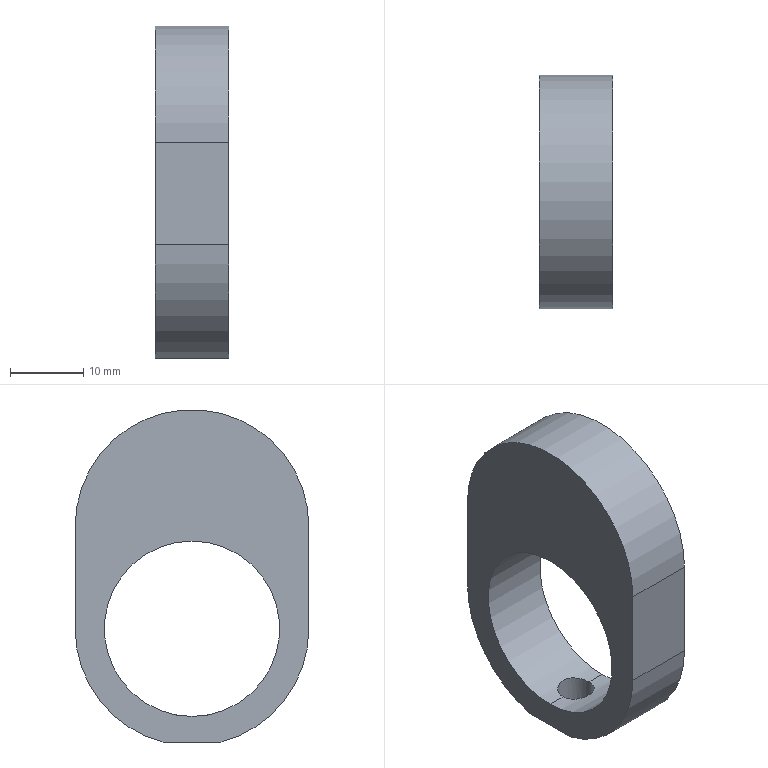Part | STEP file | 1 solid | 12 faces | box 10 x 32 x 45.5 mm | volume 7902 mm3 | cylinder 7 | plane 5 | commonest cylinder face diameters 32 x3 5 x2 24 x2
STEP:
#1=CARTESIAN_POINT('',(0.,0.,0.));
#2=DIRECTION('',(0.,0.,1.));
#3=DIRECTION('',(1.,0.,0.));
#4=AXIS2_PLACEMENT_3D('',#1,#2,#3);
#5=CARTESIAN_POINT('',(-2.5,9.488,-11.038));
#6=VERTEX_POINT('',#5);
#7=CARTESIAN_POINT('',(-2.5,9.488,-7.538));
#8=VERTEX_POINT('',#7);
#9=CARTESIAN_POINT('',(-2.5,9.488,-16.));
#10=DIRECTION('',(0.,0.,1.));
#11=VECTOR('',#10,1.);
#12=LINE('',#9,#11);
#13=CARTESIAN_POINT('',(-5.,9.488,-16.));
#14=DIRECTION('',(0.,0.,1.));
#15=DIRECTION('',(1.,0.,0.));
#16=AXIS2_PLACEMENT_3D('',#13,#14,#15);
#17=CYLINDRICAL_SURFACE('',#16,2.5);
#18=CARTESIAN_POINT('',(6.283,0.));
#19=DIRECTION('',(0.,1.));
#20=VECTOR('',#19,1.);
#21=LINE('',#18,#20);
#22=(GEOMETRIC_REPRESENTATION_CONTEXT(2)PARAMETRIC_REPRESENTATION_CONTEXT()REPRESENTATION_CONTEXT('',''));
#23=DEFINITIONAL_REPRESENTATION('',(#21),#22);
#24=PCURVE('',#17,#23);
#25=CARTESIAN_POINT('',(-5.,9.488,-16.));
#26=DIRECTION('',(0.,0.,1.));
#27=DIRECTION('',(1.,0.,0.));
#28=AXIS2_PLACEMENT_3D('',#25,#26,#27);
#29=CYLINDRICAL_SURFACE('',#28,2.5);
#30=CARTESIAN_POINT('',(0.,0.));
#31=DIRECTION('',(0.,1.));
#32=VECTOR('',#31,1.);
#33=LINE('',#30,#32);
#34=(GEOMETRIC_REPRESENTATION_CONTEXT(2)PARAMETRIC_REPRESENTATION_CONTEXT()REPRESENTATION_CONTEXT('',''));
#35=DEFINITIONAL_REPRESENTATION('',(#33),#34);
#36=PCURVE('',#29,#35);
#37=SURFACE_CURVE('',#12,(#24,#36),.PCURVE_S1.);
#38=EDGE_CURVE('',#6,#8,#37,.T.);
#39=ORIENTED_EDGE('',*,*,#38,.T.);
#40=CARTESIAN_POINT('',(-7.5,9.488,-7.538));
#41=VERTEX_POINT('',#40);
#42=CARTESIAN_POINT('',(-2.5,9.488,-7.538));
#43=CARTESIAN_POINT('',(-2.5,9.161,-7.538));
#44=CARTESIAN_POINT('',(-2.566,8.831,-7.524));
#45=CARTESIAN_POINT('',(-2.753,8.38,-7.488));
#46=CARTESIAN_POINT('',(-2.831,8.234,-7.473));
#47=CARTESIAN_POINT('',(-3.013,7.962,-7.442));
#48=CARTESIAN_POINT('',(-3.116,7.836,-7.425));
#49=CARTESIAN_POINT('',(-3.346,7.606,-7.39));
#50=CARTESIAN_POINT('',(-3.475,7.5,-7.373));
#51=CARTESIAN_POINT('',(-3.745,7.319,-7.341));
#52=CARTESIAN_POINT('',(-3.888,7.242,-7.326));
#53=CARTESIAN_POINT('',(-4.344,7.053,-7.289));
#54=CARTESIAN_POINT('',(-4.669,6.988,-7.275));
#55=CARTESIAN_POINT('',(-5.164,6.988,-7.275));
#56=CARTESIAN_POINT('',(-5.326,7.004,-7.278));
#57=CARTESIAN_POINT('',(-5.647,7.067,-7.292));
#58=CARTESIAN_POINT('',(-5.806,7.116,-7.302));
#59=CARTESIAN_POINT('',(-6.108,7.241,-7.326));
#60=CARTESIAN_POINT('',(-6.252,7.318,-7.341));
#61=CARTESIAN_POINT('',(-6.524,7.499,-7.373));
#62=CARTESIAN_POINT('',(-6.652,7.604,-7.39));
#63=CARTESIAN_POINT('',(-6.996,7.948,-7.441));
#64=CARTESIAN_POINT('',(-7.183,8.227,-7.476));
#65=CARTESIAN_POINT('',(-7.371,8.677,-7.512));
#66=CARTESIAN_POINT('',(-7.419,8.836,-7.522));
#67=CARTESIAN_POINT('',(-7.484,9.159,-7.535));
#68=CARTESIAN_POINT('',(-7.5,9.322,-7.538));
#69=CARTESIAN_POINT('',(-7.5,9.488,-7.538));
#70=B_SPLINE_CURVE_WITH_KNOTS('',3,(#42,#43,#44,#45,#46,#47,#48,#49,#50,#51,#52,#53,#54,#55,#56,#57,#58,#59,#60,#61,#62,#63,#64,#65,#66,#67,#68,#69),.UNSPECIFIED.,.F.,.F.,(4,2,2,2,2,2,2,2,2,2,2,2,2,4),(0.007838,0.008817,0.009307,0.009797,0.01029,0.01078,0.01176,0.01225,0.01273,0.01322,0.01371,0.01469,0.01518,0.01567),.UNSPECIFIED.);
#71=CARTESIAN_POINT('',(6.283,8.462));
#72=CARTESIAN_POINT('',(6.267,8.462));
#73=CARTESIAN_POINT('',(6.236,8.462));
#74=CARTESIAN_POINT('',(6.188,8.464));
#75=CARTESIAN_POINT('',(6.14,8.467));
#76=CARTESIAN_POINT('',(6.092,8.471));
#77=CARTESIAN_POINT('',(6.045,8.476));
#78=CARTESIAN_POINT('',(5.997,8.482));
#79=CARTESIAN_POINT('',(5.949,8.49));
#80=CARTESIAN_POINT('',(5.902,8.498));
#81=CARTESIAN_POINT('',(5.855,8.507));
#82=CARTESIAN_POINT('',(5.807,8.517));
#83=CARTESIAN_POINT('',(5.759,8.527));
#84=CARTESIAN_POINT('',(5.711,8.538));
#85=CARTESIAN_POINT('',(5.664,8.55));
#86=CARTESIAN_POINT('',(5.617,8.562));
#87=CARTESIAN_POINT('',(5.569,8.574));
#88=CARTESIAN_POINT('',(5.522,8.586));
#89=CARTESIAN_POINT('',(5.475,8.599));
#90=CARTESIAN_POINT('',(5.427,8.611));
#91=CARTESIAN_POINT('',(5.379,8.624));
#92=CARTESIAN_POINT('',(5.332,8.636));
#93=CARTESIAN_POINT('',(5.284,8.647));
#94=CARTESIAN_POINT('',(5.237,8.659));
#95=CARTESIAN_POINT('',(5.19,8.669));
#96=CARTESIAN_POINT('',(5.142,8.679));
#97=CARTESIAN_POINT('',(5.094,8.688));
#98=CARTESIAN_POINT('',(5.047,8.697));
#99=CARTESIAN_POINT('',(4.999,8.704));
#100=CARTESIAN_POINT('',(4.952,8.71));
#101=CARTESIAN_POINT('',(4.904,8.716));
#102=CARTESIAN_POINT('',(4.856,8.72));
#103=CARTESIAN_POINT('',(4.809,8.723));
#104=CARTESIAN_POINT('',(4.761,8.725));
#105=CARTESIAN_POINT('',(4.713,8.725));
#106=CARTESIAN_POINT('',(4.665,8.725));
#107=CARTESIAN_POINT('',(4.617,8.723));
#108=CARTESIAN_POINT('',(4.57,8.72));
#109=CARTESIAN_POINT('',(4.522,8.716));
#110=CARTESIAN_POINT('',(4.475,8.711));
#111=CARTESIAN_POINT('',(4.427,8.704));
#112=CARTESIAN_POINT('',(4.379,8.697));
#113=CARTESIAN_POINT('',(4.331,8.688));
#114=CARTESIAN_POINT('',(4.284,8.679));
#115=CARTESIAN_POINT('',(4.236,8.669));
#116=CARTESIAN_POINT('',(4.189,8.659));
#117=CARTESIAN_POINT('',(4.142,8.648));
#118=CARTESIAN_POINT('',(4.094,8.636));
#119=CARTESIAN_POINT('',(4.046,8.624));
#120=CARTESIAN_POINT('',(3.999,8.612));
#121=CARTESIAN_POINT('',(3.951,8.599));
#122=CARTESIAN_POINT('',(3.904,8.587));
#123=CARTESIAN_POINT('',(3.857,8.574));
#124=CARTESIAN_POINT('',(3.809,8.562));
#125=CARTESIAN_POINT('',(3.762,8.55));
#126=CARTESIAN_POINT('',(3.714,8.538));
#127=CARTESIAN_POINT('',(3.667,8.527));
#128=CARTESIAN_POINT('',(3.619,8.517));
#129=CARTESIAN_POINT('',(3.572,8.507));
#130=CARTESIAN_POINT('',(3.524,8.498));
#131=CARTESIAN_POINT('',(3.477,8.49));
#132=CARTESIAN_POINT('',(3.429,8.483));
#133=CARTESIAN_POINT('',(3.381,8.476));
#134=CARTESIAN_POINT('',(3.333,8.471));
#135=CARTESIAN_POINT('',(3.285,8.467));
#136=CARTESIAN_POINT('',(3.238,8.464));
#137=CARTESIAN_POINT('',(3.19,8.462));
#138=CARTESIAN_POINT('',(3.158,8.462));
#139=CARTESIAN_POINT('',(3.142,8.462));
#140=B_SPLINE_CURVE_WITH_KNOTS('',3,(#71,#72,#73,#74,#75,#76,#77,#78,#79,#80,#81,#82,#83,#84,#85,#86,#87,#88,#89,#90,#91,#92,#93,#94,#95,#96,#97,#98,#99,#100,#101,#102,#103,#104,#105,#106,#107,#108,#109,#110,#111,#112,#113,#114,#115,#116,#117,#118,#119,#120,#121,#122,#123,#124,#125,#126,#127,#128,#129,#130,#131,#132,#133,#134,#135,#136,#137,#138,#139),.UNSPECIFIED.,.F.,.F.,(4,1,1,1,1,1,1,1,1,1,1,1,1,1,1,1,1,1,1,1,1,1,1,1,1,1,1,1,1,1,1,1,1,1,1,1,1,1,1,1,1,1,1,1,1,1,1,1,1,1,1,1,1,1,1,1,1,1,1,1,1,1,1,1,1,1,4),(0.007838,0.007956,0.008075,0.008194,0.008313,0.008431,0.00855,0.008669,0.008787,0.008906,0.009025,0.009144,0.009262,0.009381,0.0095,0.009618,0.009737,0.009856,0.009975,0.01009,0.01021,0.01033,0.01045,0.01057,0.01069,0.01081,0.01092,0.01104,0.01116,0.01128,0.0114,0.01152,0.01164,0.01176,0.01187,0.01199,0.01211,0.01223,0.01235,0.01247,0.01259,0.01271,0.01282,0.01294,0.01306,0.01318,0.0133,0.01342,0.01354,0.01365,0.01377,0.01389,0.01401,0.01413,0.01425,0.01437,0.01449,0.0146,0.01472,0.01484,0.01496,0.01508,0.0152,0.01532,0.01544,0.01555,0.01567),.QUASI_UNIFORM_KNOTS.);
#141=(GEOMETRIC_REPRESENTATION_CONTEXT(2)PARAMETRIC_REPRESENTATION_CONTEXT()REPRESENTATION_CONTEXT('',''));
#142=DEFINITIONAL_REPRESENTATION('',(#140),#141);
#143=PCURVE('',#17,#142);
#144=CARTESIAN_POINT('',(-10.,9.488,4.462));
#145=DIRECTION('',(1.,0.,0.));
#146=DIRECTION('',(0.,0.,-1.));
#147=AXIS2_PLACEMENT_3D('',#144,#145,#146);
#148=CYLINDRICAL_SURFACE('',#147,12.);
#149=CARTESIAN_POINT('',(6.283,7.5));
#150=CARTESIAN_POINT('',(6.28,7.5));
#151=CARTESIAN_POINT('',(6.273,7.498));
#152=CARTESIAN_POINT('',(6.263,7.489));
#153=CARTESIAN_POINT('',(6.253,7.475));
#154=CARTESIAN_POINT('',(6.244,7.455));
#155=CARTESIAN_POINT('',(6.234,7.43));
#156=CARTESIAN_POINT('',(6.224,7.399));
#157=CARTESIAN_POINT('',(6.215,7.363));
#158=CARTESIAN_POINT('',(6.206,7.321));
#159=CARTESIAN_POINT('',(6.196,7.275));
#160=CARTESIAN_POINT('',(6.187,7.223));
#161=CARTESIAN_POINT('',(6.179,7.165));
#162=CARTESIAN_POINT('',(6.17,7.103));
#163=CARTESIAN_POINT('',(6.162,7.036));
#164=CARTESIAN_POINT('',(6.154,6.966));
#165=CARTESIAN_POINT('',(6.146,6.89));
#166=CARTESIAN_POINT('',(6.139,6.811));
#167=CARTESIAN_POINT('',(6.132,6.727));
#168=CARTESIAN_POINT('',(6.125,6.639));
#169=CARTESIAN_POINT('',(6.119,6.547));
#170=CARTESIAN_POINT('',(6.113,6.452));
#171=CARTESIAN_POINT('',(6.107,6.353));
#172=CARTESIAN_POINT('',(6.102,6.253));
#173=CARTESIAN_POINT('',(6.097,6.149));
#174=CARTESIAN_POINT('',(6.093,6.042));
#175=CARTESIAN_POINT('',(6.089,5.933));
#176=CARTESIAN_POINT('',(6.085,5.821));
#177=CARTESIAN_POINT('',(6.082,5.707));
#178=CARTESIAN_POINT('',(6.079,5.592));
#179=CARTESIAN_POINT('',(6.077,5.476));
#180=CARTESIAN_POINT('',(6.075,5.359));
#181=CARTESIAN_POINT('',(6.074,5.24));
#182=CARTESIAN_POINT('',(6.073,5.121));
#183=CARTESIAN_POINT('',(6.073,5.001));
#184=CARTESIAN_POINT('',(6.073,4.881));
#185=CARTESIAN_POINT('',(6.074,4.763));
#186=CARTESIAN_POINT('',(6.075,4.645));
#187=CARTESIAN_POINT('',(6.077,4.528));
#188=CARTESIAN_POINT('',(6.079,4.411));
#189=CARTESIAN_POINT('',(6.082,4.296));
#190=CARTESIAN_POINT('',(6.085,4.182));
#191=CARTESIAN_POINT('',(6.088,4.07));
#192=CARTESIAN_POINT('',(6.092,3.961));
#193=CARTESIAN_POINT('',(6.097,3.854));
#194=CARTESIAN_POINT('',(6.102,3.75));
#195=CARTESIAN_POINT('',(6.107,3.649));
#196=CARTESIAN_POINT('',(6.113,3.55));
#197=CARTESIAN_POINT('',(6.119,3.455));
#198=CARTESIAN_POINT('',(6.125,3.363));
#199=CARTESIAN_POINT('',(6.132,3.275));
#200=CARTESIAN_POINT('',(6.139,3.191));
#201=CARTESIAN_POINT('',(6.146,3.112));
#202=CARTESIAN_POINT('',(6.154,3.036));
#203=CARTESIAN_POINT('',(6.162,2.965));
#204=CARTESIAN_POINT('',(6.17,2.898));
#205=CARTESIAN_POINT('',(6.179,2.836));
#206=CARTESIAN_POINT('',(6.187,2.779));
#207=CARTESIAN_POINT('',(6.196,2.727));
#208=CARTESIAN_POINT('',(6.205,2.68));
#209=CARTESIAN_POINT('',(6.215,2.638));
#210=CARTESIAN_POINT('',(6.224,2.602));
#211=CARTESIAN_POINT('',(6.234,2.57));
#212=CARTESIAN_POINT('',(6.244,2.545));
#213=CARTESIAN_POINT('',(6.253,2.525));
#214=CARTESIAN_POINT('',(6.263,2.511));
#215=CARTESIAN_POINT('',(6.273,2.502));
#216=CARTESIAN_POINT('',(6.28,2.5));
#217=CARTESIAN_POINT('',(6.283,2.5));
#218=B_SPLINE_CURVE_WITH_KNOTS('',3,(#149,#150,#151,#152,#153,#154,#155,#156,#157,#158,#159,#160,#161,#162,#163,#164,#165,#166,#167,#168,#169,#170,#171,#172,#173,#174,#175,#176,#177,#178,#179,#180,#181,#182,#183,#184,#185,#186,#187,#188,#189,#190,#191,#192,#193,#194,#195,#196,#197,#198,#199,#200,#201,#202,#203,#204,#205,#206,#207,#208,#209,#210,#211,#212,#213,#214,#215,#216,#217),.UNSPECIFIED.,.F.,.F.,(4,1,1,1,1,1,1,1,1,1,1,1,1,1,1,1,1,1,1,1,1,1,1,1,1,1,1,1,1,1,1,1,1,1,1,1,1,1,1,1,1,1,1,1,1,1,1,1,1,1,1,1,1,1,1,1,1,1,1,1,1,1,1,1,1,1,4),(0.007838,0.007956,0.008075,0.008194,0.008313,0.008431,0.00855,0.008669,0.008787,0.008906,0.009025,0.009144,0.009262,0.009381,0.0095,0.009618,0.009737,0.009856,0.009975,0.01009,0.01021,0.01033,0.01045,0.01057,0.01069,0.01081,0.01092,0.01104,0.01116,0.01128,0.0114,0.01152,0.01164,0.01176,0.01187,0.01199,0.01211,0.01223,0.01235,0.01247,0.01259,0.01271,0.01282,0.01294,0.01306,0.01318,0.0133,0.01342,0.01354,0.01365,0.01377,0.01389,0.01401,0.01413,0.01425,0.01437,0.01449,0.0146,0.01472,0.01484,0.01496,0.01508,0.0152,0.01532,0.01544,0.01555,0.01567),.QUASI_UNIFORM_KNOTS.);
#219=(GEOMETRIC_REPRESENTATION_CONTEXT(2)PARAMETRIC_REPRESENTATION_CONTEXT()REPRESENTATION_CONTEXT('',''));
#220=DEFINITIONAL_REPRESENTATION('',(#218),#219);
#221=PCURVE('',#148,#220);
#222=SURFACE_CURVE('',#70,(#143,#221),.PCURVE_S1.);
#223=EDGE_CURVE('',#8,#41,#222,.T.);
#224=ORIENTED_EDGE('',*,*,#223,.T.);
#225=CARTESIAN_POINT('',(-7.5,9.488,-11.038));
#226=VERTEX_POINT('',#225);
#227=CARTESIAN_POINT('',(-7.5,9.488,-16.));
#228=DIRECTION('',(0.,0.,1.));
#229=VECTOR('',#228,1.);
#230=LINE('',#227,#229);
#231=CARTESIAN_POINT('',(3.142,0.));
#232=DIRECTION('',(0.,1.));
#233=VECTOR('',#232,1.);
#234=LINE('',#231,#233);
#235=(GEOMETRIC_REPRESENTATION_CONTEXT(2)PARAMETRIC_REPRESENTATION_CONTEXT()REPRESENTATION_CONTEXT('',''));
#236=DEFINITIONAL_REPRESENTATION('',(#234),#235);
#237=PCURVE('',#17,#236);
#238=CARTESIAN_POINT('',(3.142,0.));
#239=DIRECTION('',(0.,1.));
#240=VECTOR('',#239,1.);
#241=LINE('',#238,#240);
#242=(GEOMETRIC_REPRESENTATION_CONTEXT(2)PARAMETRIC_REPRESENTATION_CONTEXT()REPRESENTATION_CONTEXT('',''));
#243=DEFINITIONAL_REPRESENTATION('',(#241),#242);
#244=PCURVE('',#29,#243);
#245=SURFACE_CURVE('',#230,(#237,#244),.PCURVE_S1.);
#246=EDGE_CURVE('',#226,#41,#245,.T.);
#247=ORIENTED_EDGE('',*,*,#246,.F.);
#248=CARTESIAN_POINT('',(-5.,9.488,-11.038));
#249=DIRECTION('',(0.,0.,-1.));
#250=DIRECTION('',(1.,0.,0.));
#251=AXIS2_PLACEMENT_3D('',#248,#249,#250);
#252=CIRCLE('',#251,2.5);
#253=CARTESIAN_POINT('',(6.283,4.962));
#254=DIRECTION('',(-1.,0.));
#255=VECTOR('',#254,1.);
#256=LINE('',#253,#255);
#257=(GEOMETRIC_REPRESENTATION_CONTEXT(2)PARAMETRIC_REPRESENTATION_CONTEXT()REPRESENTATION_CONTEXT('',''));
#258=DEFINITIONAL_REPRESENTATION('',(#256),#257);
#259=PCURVE('',#17,#258);
#260=CARTESIAN_POINT('',(0.,0.,-11.038));
#261=DIRECTION('',(0.,0.,1.));
#262=DIRECTION('',(1.,0.,0.));
#263=AXIS2_PLACEMENT_3D('',#260,#261,#262);
#264=PLANE('',#263);
#265=CARTESIAN_POINT('',(-2.5,9.488));
#266=CARTESIAN_POINT('',(-2.5,5.158));
#267=CARTESIAN_POINT('',(-6.25,7.323));
#268=CARTESIAN_POINT('',(-10.,9.488));
#269=CARTESIAN_POINT('',(-6.25,11.653));
#270=CARTESIAN_POINT('',(-2.5,13.818));
#271=CARTESIAN_POINT('',(-2.5,9.488));
#272=(BOUNDED_CURVE()B_SPLINE_CURVE(2,(#265,#266,#267,#268,#269,#270,#271),.UNSPECIFIED.,.T.,.F.)B_SPLINE_CURVE_WITH_KNOTS((1,2,2,2,2,1),(-2.094,0.,2.094,4.189,6.283,8.378),.UNSPECIFIED.)CURVE()GEOMETRIC_REPRESENTATION_ITEM()RATIONAL_B_SPLINE_CURVE((1.,0.5,1.,0.5,1.,0.5,1.))REPRESENTATION_ITEM(''));
#273=(GEOMETRIC_REPRESENTATION_CONTEXT(2)PARAMETRIC_REPRESENTATION_CONTEXT()REPRESENTATION_CONTEXT('',''));
#274=DEFINITIONAL_REPRESENTATION('',(#272),#273);
#275=PCURVE('',#264,#274);
#276=SURFACE_CURVE('',#252,(#259,#275),.PCURVE_S1.);
#277=EDGE_CURVE('',#6,#226,#276,.T.);
#278=ORIENTED_EDGE('',*,*,#277,.F.);
#279=EDGE_LOOP('',(#39,#224,#247,#278));
#280=FACE_BOUND('',#279,.F.);
#281=ADVANCED_FACE('',(#280),#17,.F.);
#282=CARTESIAN_POINT('',(-10.,9.488,-7.538));
#283=VERTEX_POINT('',#282);
#284=CARTESIAN_POINT('',(-10.,9.488,-7.538));
#285=DIRECTION('',(1.,0.,0.));
#286=VECTOR('',#285,1.);
#287=LINE('',#284,#286);
#288=CARTESIAN_POINT('',(6.283,0.));
#289=DIRECTION('',(0.,1.));
#290=VECTOR('',#289,1.);
#291=LINE('',#288,#290);
#292=(GEOMETRIC_REPRESENTATION_CONTEXT(2)PARAMETRIC_REPRESENTATION_CONTEXT()REPRESENTATION_CONTEXT('',''));
#293=DEFINITIONAL_REPRESENTATION('',(#291),#292);
#294=PCURVE('',#148,#293);
#295=CARTESIAN_POINT('',(-10.,9.488,4.462));
#296=DIRECTION('',(1.,0.,0.));
#297=DIRECTION('',(0.,0.,-1.));
#298=AXIS2_PLACEMENT_3D('',#295,#296,#297);
#299=CYLINDRICAL_SURFACE('',#298,12.);
#300=CARTESIAN_POINT('',(0.,0.));
#301=DIRECTION('',(0.,1.));
#302=VECTOR('',#301,1.);
#303=LINE('',#300,#302);
#304=(GEOMETRIC_REPRESENTATION_CONTEXT(2)PARAMETRIC_REPRESENTATION_CONTEXT()REPRESENTATION_CONTEXT('',''));
#305=DEFINITIONAL_REPRESENTATION('',(#303),#304);
#306=PCURVE('',#299,#305);
#307=SURFACE_CURVE('',#287,(#294,#306),.PCURVE_S1.);
#308=EDGE_CURVE('',#283,#41,#307,.T.);
#309=ORIENTED_EDGE('',*,*,#308,.T.);
#310=ORIENTED_EDGE('',*,*,#223,.F.);
#311=CARTESIAN_POINT('',(0.,9.488,-7.538));
#312=VERTEX_POINT('',#311);
#313=CARTESIAN_POINT('',(-10.,9.488,-7.538));
#314=DIRECTION('',(1.,0.,0.));
#315=VECTOR('',#314,1.);
#316=LINE('',#313,#315);
#317=CARTESIAN_POINT('',(6.283,0.));
#318=DIRECTION('',(0.,1.));
#319=VECTOR('',#318,1.);
#320=LINE('',#317,#319);
#321=(GEOMETRIC_REPRESENTATION_CONTEXT(2)PARAMETRIC_REPRESENTATION_CONTEXT()REPRESENTATION_CONTEXT('',''));
#322=DEFINITIONAL_REPRESENTATION('',(#320),#321);
#323=PCURVE('',#148,#322);
#324=CARTESIAN_POINT('',(0.,0.));
#325=DIRECTION('',(0.,1.));
#326=VECTOR('',#325,1.);
#327=LINE('',#324,#326);
#328=(GEOMETRIC_REPRESENTATION_CONTEXT(2)PARAMETRIC_REPRESENTATION_CONTEXT()REPRESENTATION_CONTEXT('',''));
#329=DEFINITIONAL_REPRESENTATION('',(#327),#328);
#330=PCURVE('',#299,#329);
#331=SURFACE_CURVE('',#316,(#323,#330),.PCURVE_S1.);
#332=EDGE_CURVE('',#8,#312,#331,.T.);
#333=ORIENTED_EDGE('',*,*,#332,.T.);
#334=CARTESIAN_POINT('',(0.,9.488,16.462));
#335=VERTEX_POINT('',#334);
#336=CARTESIAN_POINT('',(0.,9.488,4.462));
#337=DIRECTION('',(1.,0.,0.));
#338=DIRECTION('',(0.,0.,-1.));
#339=AXIS2_PLACEMENT_3D('',#336,#337,#338);
#340=CIRCLE('',#339,12.);
#341=CARTESIAN_POINT('',(0.,10.));
#342=DIRECTION('',(1.,0.));
#343=VECTOR('',#342,1.);
#344=LINE('',#341,#343);
#345=(GEOMETRIC_REPRESENTATION_CONTEXT(2)PARAMETRIC_REPRESENTATION_CONTEXT()REPRESENTATION_CONTEXT('',''));
#346=DEFINITIONAL_REPRESENTATION('',(#344),#345);
#347=PCURVE('',#148,#346);
#348=CARTESIAN_POINT('',(0.,9.488,18.462));
#349=DIRECTION('',(1.,0.,0.));
#350=DIRECTION('',(0.,0.,-1.));
#351=AXIS2_PLACEMENT_3D('',#348,#349,#350);
#352=PLANE('',#351);
#353=CARTESIAN_POINT('',(14.,0.));
#354=DIRECTION('',(1.,0.));
#355=AXIS2_PLACEMENT_2D('',#353,#354);
#356=CIRCLE('',#355,12.);
#357=(GEOMETRIC_REPRESENTATION_CONTEXT(2)PARAMETRIC_REPRESENTATION_CONTEXT()REPRESENTATION_CONTEXT('',''));
#358=DEFINITIONAL_REPRESENTATION('',(#356),#357);
#359=PCURVE('',#352,#358);
#360=SURFACE_CURVE('',#340,(#347,#359),.PCURVE_S1.);
#361=EDGE_CURVE('',#335,#312,#360,.T.);
#362=ORIENTED_EDGE('',*,*,#361,.F.);
#363=CARTESIAN_POINT('',(-10.,9.488,16.462));
#364=VERTEX_POINT('',#363);
#365=CARTESIAN_POINT('',(-10.,9.488,16.462));
#366=DIRECTION('',(1.,0.,0.));
#367=VECTOR('',#366,1.);
#368=LINE('',#365,#367);
#369=CARTESIAN_POINT('',(3.142,0.));
#370=DIRECTION('',(0.,1.));
#371=VECTOR('',#370,1.);
#372=LINE('',#369,#371);
#373=(GEOMETRIC_REPRESENTATION_CONTEXT(2)PARAMETRIC_REPRESENTATION_CONTEXT()REPRESENTATION_CONTEXT('',''));
#374=DEFINITIONAL_REPRESENTATION('',(#372),#373);
#375=PCURVE('',#148,#374);
#376=CARTESIAN_POINT('',(3.142,0.));
#377=DIRECTION('',(0.,1.));
#378=VECTOR('',#377,1.);
#379=LINE('',#376,#378);
#380=(GEOMETRIC_REPRESENTATION_CONTEXT(2)PARAMETRIC_REPRESENTATION_CONTEXT()REPRESENTATION_CONTEXT('',''));
#381=DEFINITIONAL_REPRESENTATION('',(#379),#380);
#382=PCURVE('',#299,#381);
#383=SURFACE_CURVE('',#368,(#375,#382),.PCURVE_S1.);
#384=EDGE_CURVE('',#364,#335,#383,.T.);
#385=ORIENTED_EDGE('',*,*,#384,.F.);
#386=CARTESIAN_POINT('',(-10.,9.488,4.462));
#387=DIRECTION('',(1.,0.,0.));
#388=DIRECTION('',(0.,0.,-1.));
#389=AXIS2_PLACEMENT_3D('',#386,#387,#388);
#390=CIRCLE('',#389,12.);
#391=CARTESIAN_POINT('',(0.,0.));
#392=DIRECTION('',(1.,0.));
#393=VECTOR('',#392,1.);
#394=LINE('',#391,#393);
#395=(GEOMETRIC_REPRESENTATION_CONTEXT(2)PARAMETRIC_REPRESENTATION_CONTEXT()REPRESENTATION_CONTEXT('',''));
#396=DEFINITIONAL_REPRESENTATION('',(#394),#395);
#397=PCURVE('',#148,#396);
#398=CARTESIAN_POINT('',(-10.,9.488,18.462));
#399=DIRECTION('',(1.,0.,0.));
#400=DIRECTION('',(0.,0.,-1.));
#401=AXIS2_PLACEMENT_3D('',#398,#399,#400);
#402=PLANE('',#401);
#403=CARTESIAN_POINT('',(14.,0.));
#404=DIRECTION('',(1.,0.));
#405=AXIS2_PLACEMENT_2D('',#403,#404);
#406=CIRCLE('',#405,12.);
#407=(GEOMETRIC_REPRESENTATION_CONTEXT(2)PARAMETRIC_REPRESENTATION_CONTEXT()REPRESENTATION_CONTEXT('',''));
#408=DEFINITIONAL_REPRESENTATION('',(#406),#407);
#409=PCURVE('',#402,#408);
#410=SURFACE_CURVE('',#390,(#397,#409),.PCURVE_S1.);
#411=EDGE_CURVE('',#364,#283,#410,.T.);
#412=ORIENTED_EDGE('',*,*,#411,.T.);
#413=EDGE_LOOP('',(#309,#310,#333,#362,#385,#412));
#414=FACE_BOUND('',#413,.F.);
#415=ADVANCED_FACE('',(#414),#148,.F.);
#416=CARTESIAN_POINT('',(0.,5.519,-11.038));
#417=VERTEX_POINT('',#416);
#418=CARTESIAN_POINT('',(-10.,5.519,-11.038));
#419=VERTEX_POINT('',#418);
#420=CARTESIAN_POINT('',(-10.,5.519,-11.038));
#421=DIRECTION('',(-1.,0.,0.));
#422=VECTOR('',#421,1.);
#423=LINE('',#420,#422);
#424=CARTESIAN_POINT('',(-10.,9.488,4.462));
#425=DIRECTION('',(1.,0.,0.));
#426=DIRECTION('',(0.,0.,-1.));
#427=AXIS2_PLACEMENT_3D('',#424,#425,#426);
#428=CYLINDRICAL_SURFACE('',#427,16.);
#429=CARTESIAN_POINT('',(6.033,0.));
#430=DIRECTION('',(0.,-1.));
#431=VECTOR('',#430,1.);
#432=LINE('',#429,#431);
#433=(GEOMETRIC_REPRESENTATION_CONTEXT(2)PARAMETRIC_REPRESENTATION_CONTEXT()REPRESENTATION_CONTEXT('',''));
#434=DEFINITIONAL_REPRESENTATION('',(#432),#433);
#435=PCURVE('',#428,#434);
#436=CARTESIAN_POINT('',(-10.,5.519));
#437=DIRECTION('',(-1.,0.));
#438=VECTOR('',#437,1.);
#439=LINE('',#436,#438);
#440=(GEOMETRIC_REPRESENTATION_CONTEXT(2)PARAMETRIC_REPRESENTATION_CONTEXT()REPRESENTATION_CONTEXT('',''));
#441=DEFINITIONAL_REPRESENTATION('',(#439),#440);
#442=PCURVE('',#264,#441);
#443=SURFACE_CURVE('',#423,(#435,#442),.PCURVE_S1.);
#444=EDGE_CURVE('',#417,#419,#443,.T.);
#445=ORIENTED_EDGE('',*,*,#444,.F.);
#446=CARTESIAN_POINT('',(0.,-6.512,4.462));
#447=VERTEX_POINT('',#446);
#448=CARTESIAN_POINT('',(0.,9.488,4.462));
#449=DIRECTION('',(1.,0.,0.));
#450=DIRECTION('',(0.,0.,-1.));
#451=AXIS2_PLACEMENT_3D('',#448,#449,#450);
#452=CIRCLE('',#451,16.);
#453=CARTESIAN_POINT('',(0.,10.));
#454=DIRECTION('',(1.,0.));
#455=VECTOR('',#454,1.);
#456=LINE('',#453,#455);
#457=(GEOMETRIC_REPRESENTATION_CONTEXT(2)PARAMETRIC_REPRESENTATION_CONTEXT()REPRESENTATION_CONTEXT('',''));
#458=DEFINITIONAL_REPRESENTATION('',(#456),#457);
#459=PCURVE('',#428,#458);
#460=CARTESIAN_POINT('',(14.,0.));
#461=DIRECTION('',(1.,0.));
#462=AXIS2_PLACEMENT_2D('',#460,#461);
#463=CIRCLE('',#462,16.);
#464=(GEOMETRIC_REPRESENTATION_CONTEXT(2)PARAMETRIC_REPRESENTATION_CONTEXT()REPRESENTATION_CONTEXT('',''));
#465=DEFINITIONAL_REPRESENTATION('',(#463),#464);
#466=PCURVE('',#352,#465);
#467=SURFACE_CURVE('',#452,(#459,#466),.PCURVE_S1.);
#468=EDGE_CURVE('',#447,#417,#467,.T.);
#469=ORIENTED_EDGE('',*,*,#468,.F.);
#470=CARTESIAN_POINT('',(-10.,-6.512,4.462));
#471=VERTEX_POINT('',#470);
#472=CARTESIAN_POINT('',(-10.,-6.512,4.462));
#473=DIRECTION('',(1.,0.,0.));
#474=VECTOR('',#473,1.);
#475=LINE('',#472,#474);
#476=CARTESIAN_POINT('',(4.712,0.));
#477=DIRECTION('',(0.,1.));
#478=VECTOR('',#477,1.);
#479=LINE('',#476,#478);
#480=(GEOMETRIC_REPRESENTATION_CONTEXT(2)PARAMETRIC_REPRESENTATION_CONTEXT()REPRESENTATION_CONTEXT('',''));
#481=DEFINITIONAL_REPRESENTATION('',(#479),#480);
#482=PCURVE('',#428,#481);
#483=CARTESIAN_POINT('',(-10.,-6.512,18.462));
#484=DIRECTION('',(0.,-1.,0.));
#485=DIRECTION('',(0.,0.,-1.));
#486=AXIS2_PLACEMENT_3D('',#483,#484,#485);
#487=PLANE('',#486);
#488=CARTESIAN_POINT('',(14.,0.));
#489=DIRECTION('',(0.,1.));
#490=VECTOR('',#489,1.);
#491=LINE('',#488,#490);
#492=(GEOMETRIC_REPRESENTATION_CONTEXT(2)PARAMETRIC_REPRESENTATION_CONTEXT()REPRESENTATION_CONTEXT('',''));
#493=DEFINITIONAL_REPRESENTATION('',(#491),#492);
#494=PCURVE('',#487,#493);
#495=SURFACE_CURVE('',#475,(#482,#494),.PCURVE_S1.);
#496=EDGE_CURVE('',#471,#447,#495,.T.);
#497=ORIENTED_EDGE('',*,*,#496,.F.);
#498=CARTESIAN_POINT('',(-10.,9.488,4.462));
#499=DIRECTION('',(1.,0.,0.));
#500=DIRECTION('',(0.,0.,-1.));
#501=AXIS2_PLACEMENT_3D('',#498,#499,#500);
#502=CIRCLE('',#501,16.);
#503=CARTESIAN_POINT('',(0.,0.));
#504=DIRECTION('',(1.,0.));
#505=VECTOR('',#504,1.);
#506=LINE('',#503,#505);
#507=(GEOMETRIC_REPRESENTATION_CONTEXT(2)PARAMETRIC_REPRESENTATION_CONTEXT()REPRESENTATION_CONTEXT('',''));
#508=DEFINITIONAL_REPRESENTATION('',(#506),#507);
#509=PCURVE('',#428,#508);
#510=CARTESIAN_POINT('',(14.,0.));
#511=DIRECTION('',(1.,0.));
#512=AXIS2_PLACEMENT_2D('',#510,#511);
#513=CIRCLE('',#512,16.);
#514=(GEOMETRIC_REPRESENTATION_CONTEXT(2)PARAMETRIC_REPRESENTATION_CONTEXT()REPRESENTATION_CONTEXT('',''));
#515=DEFINITIONAL_REPRESENTATION('',(#513),#514);
#516=PCURVE('',#402,#515);
#517=SURFACE_CURVE('',#502,(#509,#516),.PCURVE_S1.);
#518=EDGE_CURVE('',#471,#419,#517,.T.);
#519=ORIENTED_EDGE('',*,*,#518,.T.);
#520=EDGE_LOOP('',(#445,#469,#497,#519));
#521=FACE_BOUND('',#520,.T.);
#522=ADVANCED_FACE('',(#521),#428,.T.);
#523=CARTESIAN_POINT('',(0.,25.488,18.462));
#524=VERTEX_POINT('',#523);
#525=CARTESIAN_POINT('',(0.,-6.512,18.462));
#526=VERTEX_POINT('',#525);
#527=CARTESIAN_POINT('',(0.,9.488,18.462));
#528=DIRECTION('',(1.,0.,0.));
#529=DIRECTION('',(0.,0.,-1.));
#530=AXIS2_PLACEMENT_3D('',#527,#528,#529);
#531=CIRCLE('',#530,16.);
#532=CARTESIAN_POINT('',(-10.,9.488,18.462));
#533=DIRECTION('',(1.,0.,0.));
#534=DIRECTION('',(0.,0.,-1.));
#535=AXIS2_PLACEMENT_3D('',#532,#533,#534);
#536=CYLINDRICAL_SURFACE('',#535,16.);
#537=CARTESIAN_POINT('',(0.,10.));
#538=DIRECTION('',(1.,0.));
#539=VECTOR('',#538,1.);
#540=LINE('',#537,#539);
#541=(GEOMETRIC_REPRESENTATION_CONTEXT(2)PARAMETRIC_REPRESENTATION_CONTEXT()REPRESENTATION_CONTEXT('',''));
#542=DEFINITIONAL_REPRESENTATION('',(#540),#541);
#543=PCURVE('',#536,#542);
#544=CARTESIAN_POINT('',(0.,0.));
#545=DIRECTION('',(1.,0.));
#546=AXIS2_PLACEMENT_2D('',#544,#545);
#547=CIRCLE('',#546,16.);
#548=(GEOMETRIC_REPRESENTATION_CONTEXT(2)PARAMETRIC_REPRESENTATION_CONTEXT()REPRESENTATION_CONTEXT('',''));
#549=DEFINITIONAL_REPRESENTATION('',(#547),#548);
#550=PCURVE('',#352,#549);
#551=SURFACE_CURVE('',#531,(#543,#550),.PCURVE_S1.);
#552=EDGE_CURVE('',#524,#526,#551,.T.);
#553=ORIENTED_EDGE('',*,*,#552,.F.);
#554=CARTESIAN_POINT('',(-10.,25.488,18.462));
#555=VERTEX_POINT('',#554);
#556=CARTESIAN_POINT('',(-10.,25.488,18.462));
#557=DIRECTION('',(1.,0.,0.));
#558=VECTOR('',#557,1.);
#559=LINE('',#556,#558);
#560=CARTESIAN_POINT('',(1.571,0.));
#561=DIRECTION('',(0.,1.));
#562=VECTOR('',#561,1.);
#563=LINE('',#560,#562);
#564=(GEOMETRIC_REPRESENTATION_CONTEXT(2)PARAMETRIC_REPRESENTATION_CONTEXT()REPRESENTATION_CONTEXT('',''));
#565=DEFINITIONAL_REPRESENTATION('',(#563),#564);
#566=PCURVE('',#536,#565);
#567=CARTESIAN_POINT('',(-10.,25.488,18.462));
#568=DIRECTION('',(0.,1.,0.));
#569=DIRECTION('',(0.,0.,1.));
#570=AXIS2_PLACEMENT_3D('',#567,#568,#569);
#571=PLANE('',#570);
#572=CARTESIAN_POINT('',(0.,0.));
#573=DIRECTION('',(0.,1.));
#574=VECTOR('',#573,1.);
#575=LINE('',#572,#574);
#576=(GEOMETRIC_REPRESENTATION_CONTEXT(2)PARAMETRIC_REPRESENTATION_CONTEXT()REPRESENTATION_CONTEXT('',''));
#577=DEFINITIONAL_REPRESENTATION('',(#575),#576);
#578=PCURVE('',#571,#577);
#579=SURFACE_CURVE('',#559,(#566,#578),.PCURVE_S1.);
#580=EDGE_CURVE('',#555,#524,#579,.T.);
#581=ORIENTED_EDGE('',*,*,#580,.F.);
#582=CARTESIAN_POINT('',(-10.,-6.512,18.462));
#583=VERTEX_POINT('',#582);
#584=CARTESIAN_POINT('',(-10.,9.488,18.462));
#585=DIRECTION('',(1.,0.,0.));
#586=DIRECTION('',(0.,0.,-1.));
#587=AXIS2_PLACEMENT_3D('',#584,#585,#586);
#588=CIRCLE('',#587,16.);
#589=CARTESIAN_POINT('',(0.,0.));
#590=DIRECTION('',(1.,0.));
#591=VECTOR('',#590,1.);
#592=LINE('',#589,#591);
#593=(GEOMETRIC_REPRESENTATION_CONTEXT(2)PARAMETRIC_REPRESENTATION_CONTEXT()REPRESENTATION_CONTEXT('',''));
#594=DEFINITIONAL_REPRESENTATION('',(#592),#593);
#595=PCURVE('',#536,#594);
#596=CARTESIAN_POINT('',(0.,0.));
#597=DIRECTION('',(1.,0.));
#598=AXIS2_PLACEMENT_2D('',#596,#597);
#599=CIRCLE('',#598,16.);
#600=(GEOMETRIC_REPRESENTATION_CONTEXT(2)PARAMETRIC_REPRESENTATION_CONTEXT()REPRESENTATION_CONTEXT('',''));
#601=DEFINITIONAL_REPRESENTATION('',(#599),#600);
#602=PCURVE('',#402,#601);
#603=SURFACE_CURVE('',#588,(#595,#602),.PCURVE_S1.);
#604=EDGE_CURVE('',#555,#583,#603,.T.);
#605=ORIENTED_EDGE('',*,*,#604,.T.);
#606=CARTESIAN_POINT('',(-10.,-6.512,18.462));
#607=DIRECTION('',(1.,0.,0.));
#608=VECTOR('',#607,1.);
#609=LINE('',#606,#608);
#610=CARTESIAN_POINT('',(4.712,0.));
#611=DIRECTION('',(0.,1.));
#612=VECTOR('',#611,1.);
#613=LINE('',#610,#612);
#614=(GEOMETRIC_REPRESENTATION_CONTEXT(2)PARAMETRIC_REPRESENTATION_CONTEXT()REPRESENTATION_CONTEXT('',''));
#615=DEFINITIONAL_REPRESENTATION('',(#613),#614);
#616=PCURVE('',#536,#615);
#617=CARTESIAN_POINT('',(0.,0.));
#618=DIRECTION('',(0.,1.));
#619=VECTOR('',#618,1.);
#620=LINE('',#617,#619);
#621=(GEOMETRIC_REPRESENTATION_CONTEXT(2)PARAMETRIC_REPRESENTATION_CONTEXT()REPRESENTATION_CONTEXT('',''));
#622=DEFINITIONAL_REPRESENTATION('',(#620),#621);
#623=PCURVE('',#487,#622);
#624=SURFACE_CURVE('',#609,(#616,#623),.PCURVE_S1.);
#625=EDGE_CURVE('',#583,#526,#624,.T.);
#626=ORIENTED_EDGE('',*,*,#625,.T.);
#627=EDGE_LOOP('',(#553,#581,#605,#626));
#628=FACE_BOUND('',#627,.T.);
#629=ADVANCED_FACE('',(#628),#536,.T.);
#630=CARTESIAN_POINT('',(0.,25.488,4.462));
#631=VERTEX_POINT('',#630);
#632=CARTESIAN_POINT('',(0.,25.488,18.462));
#633=DIRECTION('',(0.,0.,1.));
#634=VECTOR('',#633,1.);
#635=LINE('',#632,#634);
#636=CARTESIAN_POINT('',(0.,10.));
#637=DIRECTION('',(1.,0.));
#638=VECTOR('',#637,1.);
#639=LINE('',#636,#638);
#640=(GEOMETRIC_REPRESENTATION_CONTEXT(2)PARAMETRIC_REPRESENTATION_CONTEXT()REPRESENTATION_CONTEXT('',''));
#641=DEFINITIONAL_REPRESENTATION('',(#639),#640);
#642=PCURVE('',#571,#641);
#643=CARTESIAN_POINT('',(0.,16.));
#644=DIRECTION('',(-1.,0.));
#645=VECTOR('',#644,1.);
#646=LINE('',#643,#645);
#647=(GEOMETRIC_REPRESENTATION_CONTEXT(2)PARAMETRIC_REPRESENTATION_CONTEXT()REPRESENTATION_CONTEXT('',''));
#648=DEFINITIONAL_REPRESENTATION('',(#646),#647);
#649=PCURVE('',#352,#648);
#650=SURFACE_CURVE('',#635,(#642,#649),.PCURVE_S1.);
#651=EDGE_CURVE('',#631,#524,#650,.T.);
#652=ORIENTED_EDGE('',*,*,#651,.F.);
#653=CARTESIAN_POINT('',(-10.,25.488,4.462));
#654=VERTEX_POINT('',#653);
#655=CARTESIAN_POINT('',(-10.,25.488,4.462));
#656=DIRECTION('',(1.,0.,0.));
#657=VECTOR('',#656,1.);
#658=LINE('',#655,#657);
#659=CARTESIAN_POINT('',(-14.,0.));
#660=DIRECTION('',(0.,1.));
#661=VECTOR('',#660,1.);
#662=LINE('',#659,#661);
#663=(GEOMETRIC_REPRESENTATION_CONTEXT(2)PARAMETRIC_REPRESENTATION_CONTEXT()REPRESENTATION_CONTEXT('',''));
#664=DEFINITIONAL_REPRESENTATION('',(#662),#663);
#665=PCURVE('',#571,#664);
#666=CARTESIAN_POINT('',(-10.,9.488,4.462));
#667=DIRECTION('',(1.,0.,0.));
#668=DIRECTION('',(0.,0.,-1.));
#669=AXIS2_PLACEMENT_3D('',#666,#667,#668);
#670=CYLINDRICAL_SURFACE('',#669,16.);
#671=CARTESIAN_POINT('',(1.571,0.));
#672=DIRECTION('',(0.,1.));
#673=VECTOR('',#672,1.);
#674=LINE('',#671,#673);
#675=(GEOMETRIC_REPRESENTATION_CONTEXT(2)PARAMETRIC_REPRESENTATION_CONTEXT()REPRESENTATION_CONTEXT('',''));
#676=DEFINITIONAL_REPRESENTATION('',(#674),#675);
#677=PCURVE('',#670,#676);
#678=SURFACE_CURVE('',#658,(#665,#677),.PCURVE_S1.);
#679=EDGE_CURVE('',#654,#631,#678,.T.);
#680=ORIENTED_EDGE('',*,*,#679,.F.);
#681=CARTESIAN_POINT('',(-10.,25.488,18.462));
#682=DIRECTION('',(0.,0.,1.));
#683=VECTOR('',#682,1.);
#684=LINE('',#681,#683);
#685=CARTESIAN_POINT('',(0.,0.));
#686=DIRECTION('',(1.,0.));
#687=VECTOR('',#686,1.);
#688=LINE('',#685,#687);
#689=(GEOMETRIC_REPRESENTATION_CONTEXT(2)PARAMETRIC_REPRESENTATION_CONTEXT()REPRESENTATION_CONTEXT('',''));
#690=DEFINITIONAL_REPRESENTATION('',(#688),#689);
#691=PCURVE('',#571,#690);
#692=CARTESIAN_POINT('',(0.,16.));
#693=DIRECTION('',(-1.,0.));
#694=VECTOR('',#693,1.);
#695=LINE('',#692,#694);
#696=(GEOMETRIC_REPRESENTATION_CONTEXT(2)PARAMETRIC_REPRESENTATION_CONTEXT()REPRESENTATION_CONTEXT('',''));
#697=DEFINITIONAL_REPRESENTATION('',(#695),#696);
#698=PCURVE('',#402,#697);
#699=SURFACE_CURVE('',#684,(#691,#698),.PCURVE_S1.);
#700=EDGE_CURVE('',#654,#555,#699,.T.);
#701=ORIENTED_EDGE('',*,*,#700,.T.);
#702=ORIENTED_EDGE('',*,*,#580,.T.);
#703=EDGE_LOOP('',(#652,#680,#701,#702));
#704=FACE_BOUND('',#703,.T.);
#705=ADVANCED_FACE('',(#704),#571,.T.);
#706=CARTESIAN_POINT('',(-10.,13.456,-11.038));
#707=VERTEX_POINT('',#706);
#708=CARTESIAN_POINT('',(0.,13.456,-11.038));
#709=VERTEX_POINT('',#708);
#710=CARTESIAN_POINT('',(-10.,13.456,-11.038));
#711=DIRECTION('',(1.,0.,0.));
#712=VECTOR('',#711,1.);
#713=LINE('',#710,#712);
#714=CARTESIAN_POINT('',(0.2507,0.));
#715=DIRECTION('',(0.,1.));
#716=VECTOR('',#715,1.);
#717=LINE('',#714,#716);
#718=(GEOMETRIC_REPRESENTATION_CONTEXT(2)PARAMETRIC_REPRESENTATION_CONTEXT()REPRESENTATION_CONTEXT('',''));
#719=DEFINITIONAL_REPRESENTATION('',(#717),#718);
#720=PCURVE('',#670,#719);
#721=CARTESIAN_POINT('',(-10.,13.456));
#722=DIRECTION('',(1.,0.));
#723=VECTOR('',#722,1.);
#724=LINE('',#721,#723);
#725=(GEOMETRIC_REPRESENTATION_CONTEXT(2)PARAMETRIC_REPRESENTATION_CONTEXT()REPRESENTATION_CONTEXT('',''));
#726=DEFINITIONAL_REPRESENTATION('',(#724),#725);
#727=PCURVE('',#264,#726);
#728=SURFACE_CURVE('',#713,(#720,#727),.PCURVE_S1.);
#729=EDGE_CURVE('',#707,#709,#728,.T.);
#730=ORIENTED_EDGE('',*,*,#729,.F.);
#731=CARTESIAN_POINT('',(-10.,9.488,4.462));
#732=DIRECTION('',(1.,0.,0.));
#733=DIRECTION('',(0.,0.,-1.));
#734=AXIS2_PLACEMENT_3D('',#731,#732,#733);
#735=CIRCLE('',#734,16.);
#736=CARTESIAN_POINT('',(0.,0.));
#737=DIRECTION('',(1.,0.));
#738=VECTOR('',#737,1.);
#739=LINE('',#736,#738);
#740=(GEOMETRIC_REPRESENTATION_CONTEXT(2)PARAMETRIC_REPRESENTATION_CONTEXT()REPRESENTATION_CONTEXT('',''));
#741=DEFINITIONAL_REPRESENTATION('',(#739),#740);
#742=PCURVE('',#670,#741);
#743=CARTESIAN_POINT('',(14.,0.));
#744=DIRECTION('',(1.,0.));
#745=AXIS2_PLACEMENT_2D('',#743,#744);
#746=CIRCLE('',#745,16.);
#747=(GEOMETRIC_REPRESENTATION_CONTEXT(2)PARAMETRIC_REPRESENTATION_CONTEXT()REPRESENTATION_CONTEXT('',''));
#748=DEFINITIONAL_REPRESENTATION('',(#746),#747);
#749=PCURVE('',#402,#748);
#750=SURFACE_CURVE('',#735,(#742,#749),.PCURVE_S1.);
#751=EDGE_CURVE('',#707,#654,#750,.T.);
#752=ORIENTED_EDGE('',*,*,#751,.T.);
#753=ORIENTED_EDGE('',*,*,#679,.T.);
#754=CARTESIAN_POINT('',(0.,9.488,4.462));
#755=DIRECTION('',(1.,0.,0.));
#756=DIRECTION('',(0.,0.,-1.));
#757=AXIS2_PLACEMENT_3D('',#754,#755,#756);
#758=CIRCLE('',#757,16.);
#759=CARTESIAN_POINT('',(0.,10.));
#760=DIRECTION('',(1.,0.));
#761=VECTOR('',#760,1.);
#762=LINE('',#759,#761);
#763=(GEOMETRIC_REPRESENTATION_CONTEXT(2)PARAMETRIC_REPRESENTATION_CONTEXT()REPRESENTATION_CONTEXT('',''));
#764=DEFINITIONAL_REPRESENTATION('',(#762),#763);
#765=PCURVE('',#670,#764);
#766=CARTESIAN_POINT('',(14.,0.));
#767=DIRECTION('',(1.,0.));
#768=AXIS2_PLACEMENT_2D('',#766,#767);
#769=CIRCLE('',#768,16.);
#770=(GEOMETRIC_REPRESENTATION_CONTEXT(2)PARAMETRIC_REPRESENTATION_CONTEXT()REPRESENTATION_CONTEXT('',''));
#771=DEFINITIONAL_REPRESENTATION('',(#769),#770);
#772=PCURVE('',#352,#771);
#773=SURFACE_CURVE('',#758,(#765,#772),.PCURVE_S1.);
#774=EDGE_CURVE('',#709,#631,#773,.T.);
#775=ORIENTED_EDGE('',*,*,#774,.F.);
#776=EDGE_LOOP('',(#730,#752,#753,#775));
#777=FACE_BOUND('',#776,.T.);
#778=ADVANCED_FACE('',(#777),#670,.T.);
#779=CARTESIAN_POINT('',(0.,-6.512,18.462));
#780=DIRECTION('',(0.,0.,-1.));
#781=VECTOR('',#780,1.);
#782=LINE('',#779,#781);
#783=CARTESIAN_POINT('',(0.,10.));
#784=DIRECTION('',(1.,0.));
#785=VECTOR('',#784,1.);
#786=LINE('',#783,#785);
#787=(GEOMETRIC_REPRESENTATION_CONTEXT(2)PARAMETRIC_REPRESENTATION_CONTEXT()REPRESENTATION_CONTEXT('',''));
#788=DEFINITIONAL_REPRESENTATION('',(#786),#787);
#789=PCURVE('',#487,#788);
#790=CARTESIAN_POINT('',(0.,-16.));
#791=DIRECTION('',(1.,0.));
#792=VECTOR('',#791,1.);
#793=LINE('',#790,#792);
#794=(GEOMETRIC_REPRESENTATION_CONTEXT(2)PARAMETRIC_REPRESENTATION_CONTEXT()REPRESENTATION_CONTEXT('',''));
#795=DEFINITIONAL_REPRESENTATION('',(#793),#794);
#796=PCURVE('',#352,#795);
#797=SURFACE_CURVE('',#782,(#789,#796),.PCURVE_S1.);
#798=EDGE_CURVE('',#526,#447,#797,.T.);
#799=ORIENTED_EDGE('',*,*,#798,.F.);
#800=ORIENTED_EDGE('',*,*,#625,.F.);
#801=CARTESIAN_POINT('',(-10.,-6.512,18.462));
#802=DIRECTION('',(0.,0.,-1.));
#803=VECTOR('',#802,1.);
#804=LINE('',#801,#803);
#805=CARTESIAN_POINT('',(0.,0.));
#806=DIRECTION('',(1.,0.));
#807=VECTOR('',#806,1.);
#808=LINE('',#805,#807);
#809=(GEOMETRIC_REPRESENTATION_CONTEXT(2)PARAMETRIC_REPRESENTATION_CONTEXT()REPRESENTATION_CONTEXT('',''));
#810=DEFINITIONAL_REPRESENTATION('',(#808),#809);
#811=PCURVE('',#487,#810);
#812=CARTESIAN_POINT('',(0.,-16.));
#813=DIRECTION('',(1.,0.));
#814=VECTOR('',#813,1.);
#815=LINE('',#812,#814);
#816=(GEOMETRIC_REPRESENTATION_CONTEXT(2)PARAMETRIC_REPRESENTATION_CONTEXT()REPRESENTATION_CONTEXT('',''));
#817=DEFINITIONAL_REPRESENTATION('',(#815),#816);
#818=PCURVE('',#402,#817);
#819=SURFACE_CURVE('',#804,(#811,#818),.PCURVE_S1.);
#820=EDGE_CURVE('',#583,#471,#819,.T.);
#821=ORIENTED_EDGE('',*,*,#820,.T.);
#822=ORIENTED_EDGE('',*,*,#496,.T.);
#823=EDGE_LOOP('',(#799,#800,#821,#822));
#824=FACE_BOUND('',#823,.T.);
#825=ADVANCED_FACE('',(#824),#487,.T.);
#826=CARTESIAN_POINT('',(-10.,9.488,4.462));
#827=DIRECTION('',(1.,0.,0.));
#828=DIRECTION('',(0.,0.,-1.));
#829=AXIS2_PLACEMENT_3D('',#826,#827,#828);
#830=CIRCLE('',#829,12.);
#831=CARTESIAN_POINT('',(14.,0.));
#832=DIRECTION('',(1.,0.));
#833=AXIS2_PLACEMENT_2D('',#831,#832);
#834=CIRCLE('',#833,12.);
#835=(GEOMETRIC_REPRESENTATION_CONTEXT(2)PARAMETRIC_REPRESENTATION_CONTEXT()REPRESENTATION_CONTEXT('',''));
#836=DEFINITIONAL_REPRESENTATION('',(#834),#835);
#837=PCURVE('',#402,#836);
#838=CARTESIAN_POINT('',(0.,0.));
#839=DIRECTION('',(1.,0.));
#840=VECTOR('',#839,1.);
#841=LINE('',#838,#840);
#842=(GEOMETRIC_REPRESENTATION_CONTEXT(2)PARAMETRIC_REPRESENTATION_CONTEXT()REPRESENTATION_CONTEXT('',''));
#843=DEFINITIONAL_REPRESENTATION('',(#841),#842);
#844=PCURVE('',#299,#843);
#845=SURFACE_CURVE('',#830,(#837,#844),.PCURVE_S1.);
#846=EDGE_CURVE('',#283,#364,#845,.T.);
#847=ORIENTED_EDGE('',*,*,#846,.T.);
#848=ORIENTED_EDGE('',*,*,#411,.T.);
#849=EDGE_LOOP('',(#847,#848));
#850=FACE_BOUND('',#849,.T.);
#851=ORIENTED_EDGE('',*,*,#751,.F.);
#852=CARTESIAN_POINT('',(-10.,0.,-11.038));
#853=DIRECTION('',(0.,1.,0.));
#854=VECTOR('',#853,1.);
#855=LINE('',#852,#854);
#856=CARTESIAN_POINT('',(29.5,-9.488));
#857=DIRECTION('',(0.,1.));
#858=VECTOR('',#857,1.);
#859=LINE('',#856,#858);
#860=(GEOMETRIC_REPRESENTATION_CONTEXT(2)PARAMETRIC_REPRESENTATION_CONTEXT()REPRESENTATION_CONTEXT('',''));
#861=DEFINITIONAL_REPRESENTATION('',(#859),#860);
#862=PCURVE('',#402,#861);
#863=CARTESIAN_POINT('',(-10.,0.));
#864=DIRECTION('',(0.,1.));
#865=VECTOR('',#864,1.);
#866=LINE('',#863,#865);
#867=(GEOMETRIC_REPRESENTATION_CONTEXT(2)PARAMETRIC_REPRESENTATION_CONTEXT()REPRESENTATION_CONTEXT('',''));
#868=DEFINITIONAL_REPRESENTATION('',(#866),#867);
#869=PCURVE('',#264,#868);
#870=SURFACE_CURVE('',#855,(#862,#869),.PCURVE_S1.);
#871=EDGE_CURVE('',#419,#707,#870,.T.);
#872=ORIENTED_EDGE('',*,*,#871,.F.);
#873=ORIENTED_EDGE('',*,*,#518,.F.);
#874=ORIENTED_EDGE('',*,*,#820,.F.);
#875=ORIENTED_EDGE('',*,*,#604,.F.);
#876=ORIENTED_EDGE('',*,*,#700,.F.);
#877=EDGE_LOOP('',(#851,#872,#873,#874,#875,#876));
#878=FACE_BOUND('',#877,.T.);
#879=ADVANCED_FACE('',(#850,#878),#402,.F.);
#880=CARTESIAN_POINT('',(0.,0.,-11.038));
#881=DIRECTION('',(0.,1.,0.));
#882=VECTOR('',#881,1.);
#883=LINE('',#880,#882);
#884=CARTESIAN_POINT('',(29.5,-9.488));
#885=DIRECTION('',(0.,1.));
#886=VECTOR('',#885,1.);
#887=LINE('',#884,#886);
#888=(GEOMETRIC_REPRESENTATION_CONTEXT(2)PARAMETRIC_REPRESENTATION_CONTEXT()REPRESENTATION_CONTEXT('',''));
#889=DEFINITIONAL_REPRESENTATION('',(#887),#888);
#890=PCURVE('',#352,#889);
#891=CARTESIAN_POINT('',(0.,0.));
#892=DIRECTION('',(0.,1.));
#893=VECTOR('',#892,1.);
#894=LINE('',#891,#893);
#895=(GEOMETRIC_REPRESENTATION_CONTEXT(2)PARAMETRIC_REPRESENTATION_CONTEXT()REPRESENTATION_CONTEXT('',''));
#896=DEFINITIONAL_REPRESENTATION('',(#894),#895);
#897=PCURVE('',#264,#896);
#898=SURFACE_CURVE('',#883,(#890,#897),.PCURVE_S1.);
#899=EDGE_CURVE('',#417,#709,#898,.T.);
#900=ORIENTED_EDGE('',*,*,#899,.T.);
#901=ORIENTED_EDGE('',*,*,#774,.T.);
#902=ORIENTED_EDGE('',*,*,#651,.T.);
#903=ORIENTED_EDGE('',*,*,#552,.T.);
#904=ORIENTED_EDGE('',*,*,#798,.T.);
#905=ORIENTED_EDGE('',*,*,#468,.T.);
#906=EDGE_LOOP('',(#900,#901,#902,#903,#904,#905));
#907=FACE_BOUND('',#906,.T.);
#908=CARTESIAN_POINT('',(0.,9.488,4.462));
#909=DIRECTION('',(1.,0.,0.));
#910=DIRECTION('',(0.,0.,-1.));
#911=AXIS2_PLACEMENT_3D('',#908,#909,#910);
#912=CIRCLE('',#911,12.);
#913=CARTESIAN_POINT('',(14.,0.));
#914=DIRECTION('',(1.,0.));
#915=AXIS2_PLACEMENT_2D('',#913,#914);
#916=CIRCLE('',#915,12.);
#917=(GEOMETRIC_REPRESENTATION_CONTEXT(2)PARAMETRIC_REPRESENTATION_CONTEXT()REPRESENTATION_CONTEXT('',''));
#918=DEFINITIONAL_REPRESENTATION('',(#916),#917);
#919=PCURVE('',#352,#918);
#920=CARTESIAN_POINT('',(0.,10.));
#921=DIRECTION('',(1.,0.));
#922=VECTOR('',#921,1.);
#923=LINE('',#920,#922);
#924=(GEOMETRIC_REPRESENTATION_CONTEXT(2)PARAMETRIC_REPRESENTATION_CONTEXT()REPRESENTATION_CONTEXT('',''));
#925=DEFINITIONAL_REPRESENTATION('',(#923),#924);
#926=PCURVE('',#299,#925);
#927=SURFACE_CURVE('',#912,(#919,#926),.PCURVE_S1.);
#928=EDGE_CURVE('',#312,#335,#927,.T.);
#929=ORIENTED_EDGE('',*,*,#928,.F.);
#930=ORIENTED_EDGE('',*,*,#361,.F.);
#931=EDGE_LOOP('',(#929,#930));
#932=FACE_BOUND('',#931,.T.);
#933=ADVANCED_FACE('',(#907,#932),#352,.T.);
#934=ORIENTED_EDGE('',*,*,#928,.F.);
#935=ORIENTED_EDGE('',*,*,#332,.F.);
#936=CARTESIAN_POINT('',(-7.5,9.488,-7.538));
#937=CARTESIAN_POINT('',(-7.5,9.653,-7.538));
#938=CARTESIAN_POINT('',(-7.484,9.816,-7.535));
#939=CARTESIAN_POINT('',(-7.42,10.136,-7.522));
#940=CARTESIAN_POINT('',(-7.372,10.296,-7.512));
#941=CARTESIAN_POINT('',(-7.246,10.598,-7.488));
#942=CARTESIAN_POINT('',(-7.169,10.742,-7.473));
#943=CARTESIAN_POINT('',(-6.988,11.013,-7.442));
#944=CARTESIAN_POINT('',(-6.882,11.141,-7.424));
#945=CARTESIAN_POINT('',(-6.537,11.486,-7.373));
#946=CARTESIAN_POINT('',(-6.259,11.672,-7.338));
#947=CARTESIAN_POINT('',(-5.808,11.859,-7.302));
#948=CARTESIAN_POINT('',(-5.65,11.907,-7.292));
#949=CARTESIAN_POINT('',(-5.327,11.972,-7.278));
#950=CARTESIAN_POINT('',(-5.165,11.988,-7.275));
#951=CARTESIAN_POINT('',(-4.837,11.988,-7.275));
#952=CARTESIAN_POINT('',(-4.671,11.972,-7.278));
#953=CARTESIAN_POINT('',(-4.35,11.907,-7.292));
#954=CARTESIAN_POINT('',(-4.194,11.86,-7.302));
#955=CARTESIAN_POINT('',(-3.891,11.734,-7.326));
#956=CARTESIAN_POINT('',(-3.745,11.656,-7.341));
#957=CARTESIAN_POINT('',(-3.475,11.475,-7.373));
#958=CARTESIAN_POINT('',(-3.348,11.372,-7.39));
#959=CARTESIAN_POINT('',(-3.116,11.139,-7.425));
#960=CARTESIAN_POINT('',(-3.013,11.014,-7.442));
#961=CARTESIAN_POINT('',(-2.832,10.743,-7.473));
#962=CARTESIAN_POINT('',(-2.753,10.597,-7.488));
#963=CARTESIAN_POINT('',(-2.628,10.295,-7.512));
#964=CARTESIAN_POINT('',(-2.581,10.139,-7.522));
#965=CARTESIAN_POINT('',(-2.516,9.817,-7.535));
#966=CARTESIAN_POINT('',(-2.5,9.651,-7.538));
#967=CARTESIAN_POINT('',(-2.5,9.488,-7.538));
#968=B_SPLINE_CURVE_WITH_KNOTS('',3,(#936,#937,#938,#939,#940,#941,#942,#943,#944,#945,#946,#947,#948,#949,#950,#951,#952,#953,#954,#955,#956,#957,#958,#959,#960,#961,#962,#963,#964,#965,#966,#967),.UNSPECIFIED.,.F.,.F.,(4,2,2,2,2,2,2,2,2,2,2,2,2,2,2,4),(0.,0.0004899,0.0009797,0.00147,0.001959,0.002939,0.003429,0.003919,0.004409,0.004899,0.005388,0.005878,0.006368,0.006858,0.007348,0.007838),.UNSPECIFIED.);
#969=CARTESIAN_POINT('',(0.,2.5));
#970=CARTESIAN_POINT('',(0.003347,2.5));
#971=CARTESIAN_POINT('',(0.01001,2.502));
#972=CARTESIAN_POINT('',(0.01993,2.51));
#973=CARTESIAN_POINT('',(0.02977,2.525));
#974=CARTESIAN_POINT('',(0.03952,2.544));
#975=CARTESIAN_POINT('',(0.04922,2.57));
#976=CARTESIAN_POINT('',(0.05885,2.601));
#977=CARTESIAN_POINT('',(0.06837,2.637));
#978=CARTESIAN_POINT('',(0.07773,2.679));
#979=CARTESIAN_POINT('',(0.08687,2.726));
#980=CARTESIAN_POINT('',(0.09579,2.778));
#981=CARTESIAN_POINT('',(0.1045,2.835));
#982=CARTESIAN_POINT('',(0.113,2.896));
#983=CARTESIAN_POINT('',(0.1212,2.963));
#984=CARTESIAN_POINT('',(0.1292,3.035));
#985=CARTESIAN_POINT('',(0.137,3.111));
#986=CARTESIAN_POINT('',(0.1444,3.191));
#987=CARTESIAN_POINT('',(0.1514,3.274));
#988=CARTESIAN_POINT('',(0.1581,3.362));
#989=CARTESIAN_POINT('',(0.1645,3.454));
#990=CARTESIAN_POINT('',(0.1705,3.549));
#991=CARTESIAN_POINT('',(0.1762,3.647));
#992=CARTESIAN_POINT('',(0.1814,3.749));
#993=CARTESIAN_POINT('',(0.1863,3.853));
#994=CARTESIAN_POINT('',(0.1907,3.96));
#995=CARTESIAN_POINT('',(0.1946,4.069));
#996=CARTESIAN_POINT('',(0.1982,4.18));
#997=CARTESIAN_POINT('',(0.2013,4.293));
#998=CARTESIAN_POINT('',(0.2039,4.409));
#999=CARTESIAN_POINT('',(0.2061,4.526));
#1000=CARTESIAN_POINT('',(0.2078,4.644));
#1001=CARTESIAN_POINT('',(0.209,4.762));
#1002=CARTESIAN_POINT('',(0.2097,4.88));
#1003=CARTESIAN_POINT('',(0.21,4.999));
#1004=CARTESIAN_POINT('',(0.2097,5.118));
#1005=CARTESIAN_POINT('',(0.209,5.238));
#1006=CARTESIAN_POINT('',(0.2078,5.357));
#1007=CARTESIAN_POINT('',(0.2061,5.475));
#1008=CARTESIAN_POINT('',(0.2039,5.591));
#1009=CARTESIAN_POINT('',(0.2013,5.706));
#1010=CARTESIAN_POINT('',(0.1982,5.819));
#1011=CARTESIAN_POINT('',(0.1947,5.93));
#1012=CARTESIAN_POINT('',(0.1907,6.04));
#1013=CARTESIAN_POINT('',(0.1863,6.147));
#1014=CARTESIAN_POINT('',(0.1814,6.252));
#1015=CARTESIAN_POINT('',(0.1762,6.353));
#1016=CARTESIAN_POINT('',(0.1706,6.451));
#1017=CARTESIAN_POINT('',(0.1646,6.546));
#1018=CARTESIAN_POINT('',(0.1582,6.638));
#1019=CARTESIAN_POINT('',(0.1514,6.726));
#1020=CARTESIAN_POINT('',(0.1443,6.81));
#1021=CARTESIAN_POINT('',(0.1369,6.89));
#1022=CARTESIAN_POINT('',(0.1292,6.966));
#1023=CARTESIAN_POINT('',(0.1213,7.036));
#1024=CARTESIAN_POINT('',(0.1131,7.103));
#1025=CARTESIAN_POINT('',(0.1045,7.165));
#1026=CARTESIAN_POINT('',(0.09577,7.222));
#1027=CARTESIAN_POINT('',(0.08678,7.274));
#1028=CARTESIAN_POINT('',(0.07762,7.321));
#1029=CARTESIAN_POINT('',(0.06833,7.363));
#1030=CARTESIAN_POINT('',(0.05891,7.399));
#1031=CARTESIAN_POINT('',(0.04935,7.43));
#1032=CARTESIAN_POINT('',(0.03966,7.455));
#1033=CARTESIAN_POINT('',(0.02982,7.475));
#1034=CARTESIAN_POINT('',(0.01989,7.489));
#1035=CARTESIAN_POINT('',(0.009929,7.498));
#1036=CARTESIAN_POINT('',(0.003301,7.5));
#1037=CARTESIAN_POINT('',(0.,7.5));
#1038=B_SPLINE_CURVE_WITH_KNOTS('',3,(#969,#970,#971,#972,#973,#974,#975,#976,#977,#978,#979,#980,#981,#982,#983,#984,#985,#986,#987,#988,#989,#990,#991,#992,#993,#994,#995,#996,#997,#998,#999,#1000,#1001,#1002,#1003,#1004,#1005,#1006,#1007,#1008,#1009,#1010,#1011,#1012,#1013,#1014,#1015,#1016,#1017,#1018,#1019,#1020,#1021,#1022,#1023,#1024,#1025,#1026,#1027,#1028,#1029,#1030,#1031,#1032,#1033,#1034,#1035,#1036,#1037),.UNSPECIFIED.,.F.,.F.,(4,1,1,1,1,1,1,1,1,1,1,1,1,1,1,1,1,1,1,1,1,1,1,1,1,1,1,1,1,1,1,1,1,1,1,1,1,1,1,1,1,1,1,1,1,1,1,1,1,1,1,1,1,1,1,1,1,1,1,1,1,1,1,1,1,1,4),(0.,0.0001188,0.0002375,0.0003563,0.000475,0.0005938,0.0007125,0.0008313,0.00095,0.001069,0.001188,0.001306,0.001425,0.001544,0.001663,0.001781,0.0019,0.002019,0.002138,0.002256,0.002375,0.002494,0.002613,0.002731,0.00285,0.002969,0.003088,0.003206,0.003325,0.003444,0.003563,0.003681,0.0038,0.003919,0.004038,0.004156,0.004275,0.004394,0.004513,0.004631,0.00475,0.004869,0.004988,0.005106,0.005225,0.005344,0.005463,0.005581,0.0057,0.005819,0.005938,0.006056,0.006175,0.006294,0.006413,0.006531,0.00665,0.006769,0.006888,0.007006,0.007125,0.007244,0.007363,0.007481,0.0076,0.007719,0.007838),.QUASI_UNIFORM_KNOTS.);
#1039=(GEOMETRIC_REPRESENTATION_CONTEXT(2)PARAMETRIC_REPRESENTATION_CONTEXT()REPRESENTATION_CONTEXT('',''));
#1040=DEFINITIONAL_REPRESENTATION('',(#1038),#1039);
#1041=PCURVE('',#299,#1040);
#1042=CARTESIAN_POINT('',(3.142,8.462));
#1043=CARTESIAN_POINT('',(3.126,8.462));
#1044=CARTESIAN_POINT('',(3.094,8.462));
#1045=CARTESIAN_POINT('',(3.046,8.464));
#1046=CARTESIAN_POINT('',(2.998,8.467));
#1047=CARTESIAN_POINT('',(2.951,8.471));
#1048=CARTESIAN_POINT('',(2.903,8.476));
#1049=CARTESIAN_POINT('',(2.855,8.482));
#1050=CARTESIAN_POINT('',(2.808,8.49));
#1051=CARTESIAN_POINT('',(2.76,8.498));
#1052=CARTESIAN_POINT('',(2.712,8.507));
#1053=CARTESIAN_POINT('',(2.665,8.517));
#1054=CARTESIAN_POINT('',(2.617,8.527));
#1055=CARTESIAN_POINT('',(2.57,8.538));
#1056=CARTESIAN_POINT('',(2.523,8.55));
#1057=CARTESIAN_POINT('',(2.475,8.562));
#1058=CARTESIAN_POINT('',(2.427,8.574));
#1059=CARTESIAN_POINT('',(2.38,8.587));
#1060=CARTESIAN_POINT('',(2.332,8.599));
#1061=CARTESIAN_POINT('',(2.285,8.611));
#1062=CARTESIAN_POINT('',(2.237,8.624));
#1063=CARTESIAN_POINT('',(2.19,8.636));
#1064=CARTESIAN_POINT('',(2.142,8.647));
#1065=CARTESIAN_POINT('',(2.095,8.659));
#1066=CARTESIAN_POINT('',(2.047,8.669));
#1067=CARTESIAN_POINT('',(2.,8.679));
#1068=CARTESIAN_POINT('',(1.952,8.688));
#1069=CARTESIAN_POINT('',(1.905,8.697));
#1070=CARTESIAN_POINT('',(1.857,8.704));
#1071=CARTESIAN_POINT('',(1.809,8.71));
#1072=CARTESIAN_POINT('',(1.761,8.716));
#1073=CARTESIAN_POINT('',(1.714,8.72));
#1074=CARTESIAN_POINT('',(1.666,8.723));
#1075=CARTESIAN_POINT('',(1.619,8.725));
#1076=CARTESIAN_POINT('',(1.571,8.725));
#1077=CARTESIAN_POINT('',(1.523,8.725));
#1078=CARTESIAN_POINT('',(1.476,8.723));
#1079=CARTESIAN_POINT('',(1.428,8.72));
#1080=CARTESIAN_POINT('',(1.38,8.716));
#1081=CARTESIAN_POINT('',(1.332,8.71));
#1082=CARTESIAN_POINT('',(1.285,8.704));
#1083=CARTESIAN_POINT('',(1.237,8.697));
#1084=CARTESIAN_POINT('',(1.19,8.688));
#1085=CARTESIAN_POINT('',(1.142,8.679));
#1086=CARTESIAN_POINT('',(1.094,8.669));
#1087=CARTESIAN_POINT('',(1.047,8.659));
#1088=CARTESIAN_POINT('',(0.999,8.647));
#1089=CARTESIAN_POINT('',(0.9517,8.636));
#1090=CARTESIAN_POINT('',(0.9043,8.624));
#1091=CARTESIAN_POINT('',(0.8568,8.612));
#1092=CARTESIAN_POINT('',(0.8092,8.599));
#1093=CARTESIAN_POINT('',(0.7614,8.586));
#1094=CARTESIAN_POINT('',(0.7139,8.574));
#1095=CARTESIAN_POINT('',(0.6666,8.562));
#1096=CARTESIAN_POINT('',(0.6194,8.55));
#1097=CARTESIAN_POINT('',(0.5721,8.538));
#1098=CARTESIAN_POINT('',(0.5245,8.527));
#1099=CARTESIAN_POINT('',(0.4767,8.517));
#1100=CARTESIAN_POINT('',(0.4289,8.507));
#1101=CARTESIAN_POINT('',(0.3812,8.498));
#1102=CARTESIAN_POINT('',(0.3338,8.49));
#1103=CARTESIAN_POINT('',(0.2864,8.482));
#1104=CARTESIAN_POINT('',(0.239,8.476));
#1105=CARTESIAN_POINT('',(0.1914,8.471));
#1106=CARTESIAN_POINT('',(0.1435,8.467));
#1107=CARTESIAN_POINT('',(0.09558,8.464));
#1108=CARTESIAN_POINT('',(0.04766,8.462));
#1109=CARTESIAN_POINT('',(0.01585,8.462));
#1110=CARTESIAN_POINT('',(0.,8.462));
#1111=B_SPLINE_CURVE_WITH_KNOTS('',3,(#1042,#1043,#1044,#1045,#1046,#1047,#1048,#1049,#1050,#1051,#1052,#1053,#1054,#1055,#1056,#1057,#1058,#1059,#1060,#1061,#1062,#1063,#1064,#1065,#1066,#1067,#1068,#1069,#1070,#1071,#1072,#1073,#1074,#1075,#1076,#1077,#1078,#1079,#1080,#1081,#1082,#1083,#1084,#1085,#1086,#1087,#1088,#1089,#1090,#1091,#1092,#1093,#1094,#1095,#1096,#1097,#1098,#1099,#1100,#1101,#1102,#1103,#1104,#1105,#1106,#1107,#1108,#1109,#1110),.UNSPECIFIED.,.F.,.F.,(4,1,1,1,1,1,1,1,1,1,1,1,1,1,1,1,1,1,1,1,1,1,1,1,1,1,1,1,1,1,1,1,1,1,1,1,1,1,1,1,1,1,1,1,1,1,1,1,1,1,1,1,1,1,1,1,1,1,1,1,1,1,1,1,1,1,4),(0.,0.0001188,0.0002375,0.0003563,0.000475,0.0005938,0.0007125,0.0008313,0.00095,0.001069,0.001188,0.001306,0.001425,0.001544,0.001663,0.001781,0.0019,0.002019,0.002138,0.002256,0.002375,0.002494,0.002613,0.002731,0.00285,0.002969,0.003088,0.003206,0.003325,0.003444,0.003563,0.003681,0.0038,0.003919,0.004038,0.004156,0.004275,0.004394,0.004513,0.004631,0.00475,0.004869,0.004988,0.005106,0.005225,0.005344,0.005463,0.005581,0.0057,0.005819,0.005938,0.006056,0.006175,0.006294,0.006413,0.006531,0.00665,0.006769,0.006888,0.007006,0.007125,0.007244,0.007363,0.007481,0.0076,0.007719,0.007838),.QUASI_UNIFORM_KNOTS.);
#1112=(GEOMETRIC_REPRESENTATION_CONTEXT(2)PARAMETRIC_REPRESENTATION_CONTEXT()REPRESENTATION_CONTEXT('',''));
#1113=DEFINITIONAL_REPRESENTATION('',(#1111),#1112);
#1114=PCURVE('',#29,#1113);
#1115=SURFACE_CURVE('',#968,(#1041,#1114),.PCURVE_S1.);
#1116=EDGE_CURVE('',#41,#8,#1115,.T.);
#1117=ORIENTED_EDGE('',*,*,#1116,.F.);
#1118=ORIENTED_EDGE('',*,*,#308,.F.);
#1119=ORIENTED_EDGE('',*,*,#846,.T.);
#1120=ORIENTED_EDGE('',*,*,#384,.T.);
#1121=EDGE_LOOP('',(#934,#935,#1117,#1118,#1119,#1120));
#1122=FACE_BOUND('',#1121,.F.);
#1123=ADVANCED_FACE('',(#1122),#299,.F.);
#1124=ORIENTED_EDGE('',*,*,#1116,.T.);
#1125=ORIENTED_EDGE('',*,*,#38,.F.);
#1126=CARTESIAN_POINT('',(-5.,9.488,-11.038));
#1127=DIRECTION('',(0.,0.,-1.));
#1128=DIRECTION('',(1.,0.,0.));
#1129=AXIS2_PLACEMENT_3D('',#1126,#1127,#1128);
#1130=CIRCLE('',#1129,2.5);
#1131=CARTESIAN_POINT('',(6.283,4.962));
#1132=DIRECTION('',(-1.,0.));
#1133=VECTOR('',#1132,1.);
#1134=LINE('',#1131,#1133);
#1135=(GEOMETRIC_REPRESENTATION_CONTEXT(2)PARAMETRIC_REPRESENTATION_CONTEXT()REPRESENTATION_CONTEXT('',''));
#1136=DEFINITIONAL_REPRESENTATION('',(#1134),#1135);
#1137=PCURVE('',#29,#1136);
#1138=CARTESIAN_POINT('',(-2.5,9.488));
#1139=CARTESIAN_POINT('',(-2.5,5.158));
#1140=CARTESIAN_POINT('',(-6.25,7.323));
#1141=CARTESIAN_POINT('',(-10.,9.488));
#1142=CARTESIAN_POINT('',(-6.25,11.653));
#1143=CARTESIAN_POINT('',(-2.5,13.818));
#1144=CARTESIAN_POINT('',(-2.5,9.488));
#1145=(BOUNDED_CURVE()B_SPLINE_CURVE(2,(#1138,#1139,#1140,#1141,#1142,#1143,#1144),.UNSPECIFIED.,.T.,.F.)B_SPLINE_CURVE_WITH_KNOTS((1,2,2,2,2,1),(-2.094,0.,2.094,4.189,6.283,8.378),.UNSPECIFIED.)CURVE()GEOMETRIC_REPRESENTATION_ITEM()RATIONAL_B_SPLINE_CURVE((1.,0.5,1.,0.5,1.,0.5,1.))REPRESENTATION_ITEM(''));
#1146=(GEOMETRIC_REPRESENTATION_CONTEXT(2)PARAMETRIC_REPRESENTATION_CONTEXT()REPRESENTATION_CONTEXT('',''));
#1147=DEFINITIONAL_REPRESENTATION('',(#1145),#1146);
#1148=PCURVE('',#264,#1147);
#1149=SURFACE_CURVE('',#1130,(#1137,#1148),.PCURVE_S1.);
#1150=EDGE_CURVE('',#226,#6,#1149,.T.);
#1151=ORIENTED_EDGE('',*,*,#1150,.F.);
#1152=ORIENTED_EDGE('',*,*,#246,.T.);
#1153=EDGE_LOOP('',(#1124,#1125,#1151,#1152));
#1154=FACE_BOUND('',#1153,.F.);
#1155=ADVANCED_FACE('',(#1154),#29,.F.);
#1156=ORIENTED_EDGE('',*,*,#444,.T.);
#1157=ORIENTED_EDGE('',*,*,#871,.T.);
#1158=ORIENTED_EDGE('',*,*,#729,.T.);
#1159=ORIENTED_EDGE('',*,*,#899,.F.);
#1160=EDGE_LOOP('',(#1156,#1157,#1158,#1159));
#1161=FACE_BOUND('',#1160,.T.);
#1162=ORIENTED_EDGE('',*,*,#277,.F.);
#1163=ORIENTED_EDGE('',*,*,#1150,.F.);
#1164=EDGE_LOOP('',(#1162,#1163));
#1165=FACE_BOUND('',#1164,.T.);
#1166=ADVANCED_FACE('',(#1161,#1165),#264,.F.);
#1167=CLOSED_SHELL('',(#281,#415,#522,#629,#705,#778,#825,#879,#933,#1123,#1155,#1166));
#1168=MANIFOLD_SOLID_BREP('',#1167);
#1169=(LENGTH_UNIT()NAMED_UNIT(*)SI_UNIT(.MILLI.,.METRE.));
#1170=UNCERTAINTY_MEASURE_WITH_UNIT(LENGTH_MEASURE(0.00002),#1169,'','');
#1171=(NAMED_UNIT(*)PLANE_ANGLE_UNIT()SI_UNIT($,.RADIAN.));
#1172=(NAMED_UNIT(*)SI_UNIT($,.STERADIAN.)SOLID_ANGLE_UNIT());
#1173=(GEOMETRIC_REPRESENTATION_CONTEXT(3)GLOBAL_UNCERTAINTY_ASSIGNED_CONTEXT((#1170))GLOBAL_UNIT_ASSIGNED_CONTEXT((#1169,#1171,#1172))REPRESENTATION_CONTEXT('',''));
#1174=ADVANCED_BREP_SHAPE_REPRESENTATION('',(#4,#1168),#1173);